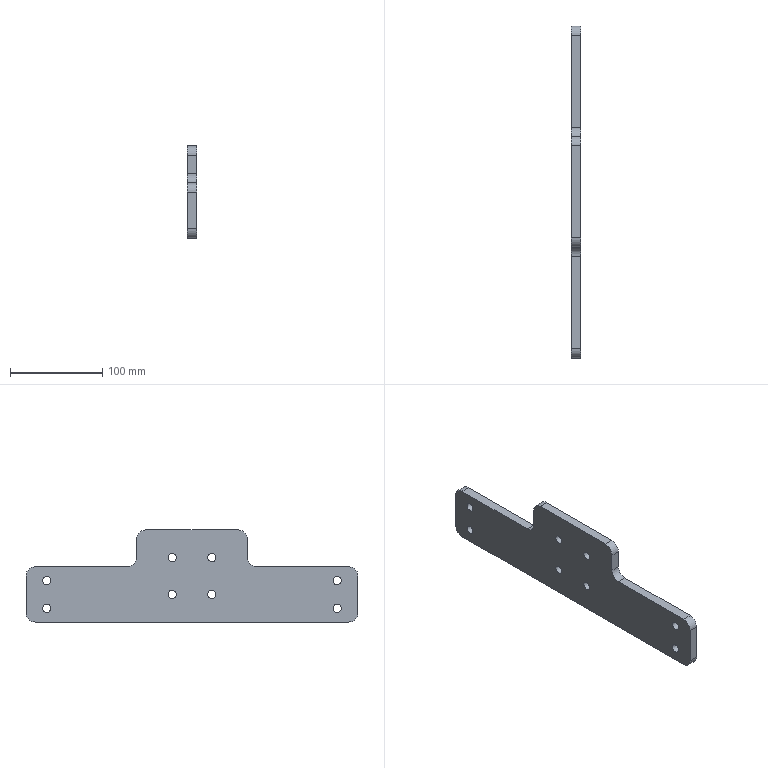Part | STEP file | SN10_013_004_PLACA | 1 solid | 26 faces | box 10 x 360 x 100 mm | volume 258052 mm3 | cylinder 16 | plane 10 | commonest cylinder face diameters 9 x8 20 x8